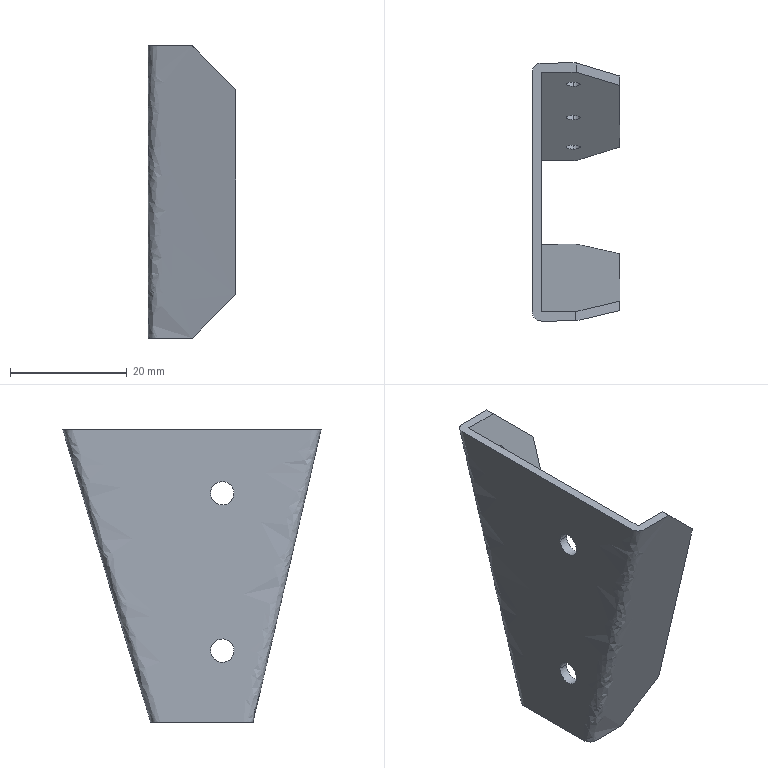Part | SolidWorks | features BaseBody 1 | 1 solid | 22 faces | box 15.009 x 44.16 x 50 mm | volume 4853 mm3 | cylinder 10 | spline 10 | plane 2 | commonest cylinder face diameters 2.4 x6 4 x4